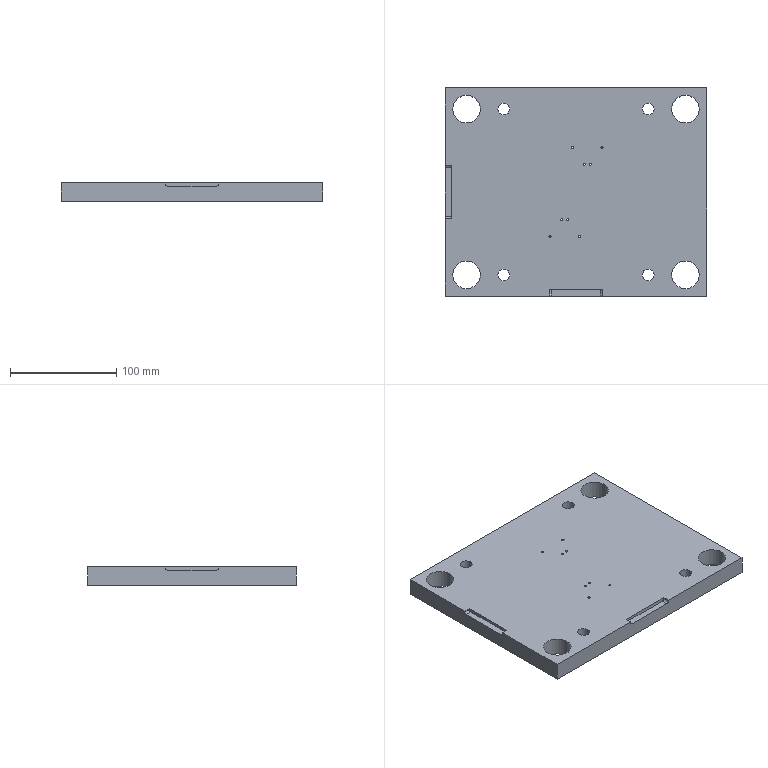Part | STEP file | 4 | 1 solid | 64 faces | box 246 x 196 x 17 mm | volume 768629 mm3 | cylinder 44 | plane 16 | cone 4 | commonest cylinder face diameters 2 x16 11 x8 26 x8 4 x4 8.5 x4 18 x4